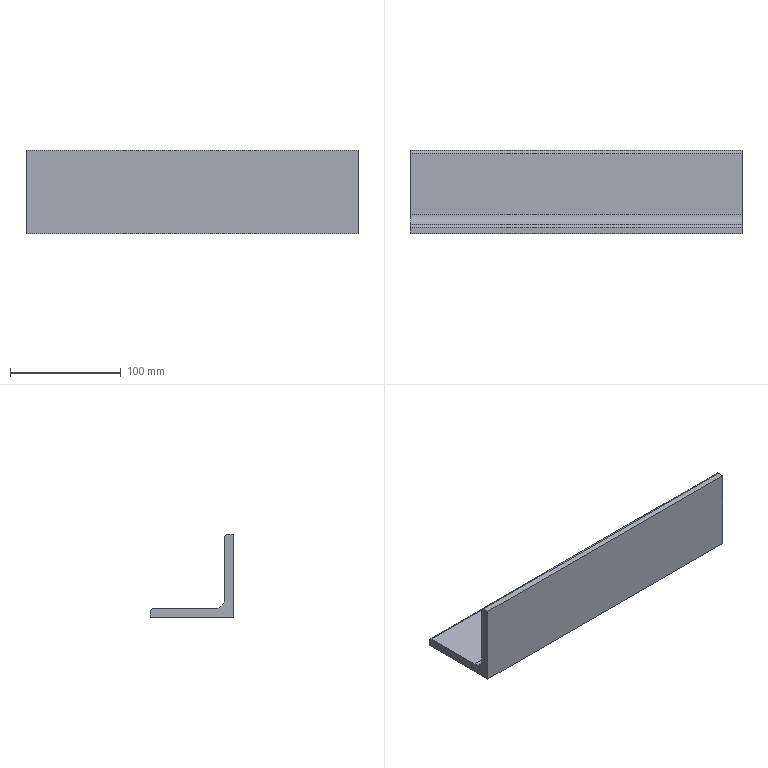Part | SolidWorks | features Extrusion 1 | 1 solid | 11 faces | box 300 x 75 x 75 mm | volume 345099 mm3 | plane 8 | cylinder 3 | commonest cylinder face diameters 5.333 x2 18 x1
STEP:
#1=CARTESIAN_POINT('',(0.,5.333,75.));
#2=VERTEX_POINT('',#1);
#3=CARTESIAN_POINT('',(0.,0.,75.));
#4=VERTEX_POINT('',#3);
#5=CARTESIAN_POINT('',(0.,0.,75.));
#6=DIRECTION('',(0.,-1.,0.));
#7=VECTOR('',#6,1000.);
#8=LINE('',#5,#7);
#9=EDGE_CURVE('',#2,#4,#8,.T.);
#10=ORIENTED_EDGE('',*,*,#9,.T.);
#11=CARTESIAN_POINT('',(300.,0.,75.));
#12=VERTEX_POINT('',#11);
#13=CARTESIAN_POINT('',(300.,0.,75.));
#14=DIRECTION('',(-1.,0.,0.));
#15=VECTOR('',#14,1000.);
#16=LINE('',#13,#15);
#17=EDGE_CURVE('',#12,#4,#16,.T.);
#18=ORIENTED_EDGE('',*,*,#17,.F.);
#19=CARTESIAN_POINT('',(300.,5.333,75.));
#20=VERTEX_POINT('',#19);
#21=CARTESIAN_POINT('',(300.,0.,75.));
#22=DIRECTION('',(0.,-1.,0.));
#23=VECTOR('',#22,1000.);
#24=LINE('',#21,#23);
#25=EDGE_CURVE('',#20,#12,#24,.T.);
#26=ORIENTED_EDGE('',*,*,#25,.F.);
#27=CARTESIAN_POINT('',(300.,5.333,75.));
#28=DIRECTION('',(-1.,0.,0.));
#29=VECTOR('',#28,1000.);
#30=LINE('',#27,#29);
#31=EDGE_CURVE('',#20,#2,#30,.T.);
#32=ORIENTED_EDGE('',*,*,#31,.T.);
#33=EDGE_LOOP('',(#10,#18,#26,#32));
#34=FACE_OUTER_BOUND('',#33,.T.);
#35=CARTESIAN_POINT('',(300.,0.,75.));
#36=DIRECTION('',(0.,0.,-1.));
#37=DIRECTION('',(-1.,0.,0.));
#38=AXIS2_PLACEMENT_3D('',#35,#36,#37);
#39=PLANE('',#38);
#40=ADVANCED_FACE('',(#34),#39,.F.);
#41=CARTESIAN_POINT('',(0.,0.,0.));
#42=VERTEX_POINT('',#41);
#43=CARTESIAN_POINT('',(0.,0.,75.));
#44=DIRECTION('',(0.,0.,-1.));
#45=VECTOR('',#44,1000.);
#46=LINE('',#43,#45);
#47=EDGE_CURVE('',#4,#42,#46,.T.);
#48=ORIENTED_EDGE('',*,*,#47,.T.);
#49=CARTESIAN_POINT('',(300.,0.,0.));
#50=VERTEX_POINT('',#49);
#51=CARTESIAN_POINT('',(300.,0.,0.));
#52=DIRECTION('',(-1.,0.,0.));
#53=VECTOR('',#52,1000.);
#54=LINE('',#51,#53);
#55=EDGE_CURVE('',#50,#42,#54,.T.);
#56=ORIENTED_EDGE('',*,*,#55,.F.);
#57=CARTESIAN_POINT('',(300.,0.,75.));
#58=DIRECTION('',(0.,0.,-1.));
#59=VECTOR('',#58,1000.);
#60=LINE('',#57,#59);
#61=EDGE_CURVE('',#12,#50,#60,.T.);
#62=ORIENTED_EDGE('',*,*,#61,.F.);
#63=ORIENTED_EDGE('',*,*,#17,.T.);
#64=EDGE_LOOP('',(#48,#56,#62,#63));
#65=FACE_OUTER_BOUND('',#64,.T.);
#66=CARTESIAN_POINT('',(300.,0.,75.));
#67=DIRECTION('',(0.,1.,0.));
#68=DIRECTION('',(0.,0.,1.));
#69=AXIS2_PLACEMENT_3D('',#66,#67,#68);
#70=PLANE('',#69);
#71=ADVANCED_FACE('',(#65),#70,.F.);
#72=CARTESIAN_POINT('',(0.,75.,0.));
#73=VERTEX_POINT('',#72);
#74=CARTESIAN_POINT('',(0.,0.,0.));
#75=DIRECTION('',(0.,1.,0.));
#76=VECTOR('',#75,1000.);
#77=LINE('',#74,#76);
#78=EDGE_CURVE('',#42,#73,#77,.T.);
#79=ORIENTED_EDGE('',*,*,#78,.T.);
#80=CARTESIAN_POINT('',(300.,75.,0.));
#81=VERTEX_POINT('',#80);
#82=CARTESIAN_POINT('',(300.,75.,0.));
#83=DIRECTION('',(-1.,0.,0.));
#84=VECTOR('',#83,1000.);
#85=LINE('',#82,#84);
#86=EDGE_CURVE('',#81,#73,#85,.T.);
#87=ORIENTED_EDGE('',*,*,#86,.F.);
#88=CARTESIAN_POINT('',(300.,0.,0.));
#89=DIRECTION('',(0.,1.,0.));
#90=VECTOR('',#89,1000.);
#91=LINE('',#88,#90);
#92=EDGE_CURVE('',#50,#81,#91,.T.);
#93=ORIENTED_EDGE('',*,*,#92,.F.);
#94=ORIENTED_EDGE('',*,*,#55,.T.);
#95=EDGE_LOOP('',(#79,#87,#93,#94));
#96=FACE_OUTER_BOUND('',#95,.T.);
#97=CARTESIAN_POINT('',(300.,0.,0.));
#98=DIRECTION('',(0.,0.,1.));
#99=DIRECTION('',(1.,0.,0.));
#100=AXIS2_PLACEMENT_3D('',#97,#98,#99);
#101=PLANE('',#100);
#102=ADVANCED_FACE('',(#96),#101,.F.);
#103=CARTESIAN_POINT('',(0.,75.,5.333));
#104=VERTEX_POINT('',#103);
#105=CARTESIAN_POINT('',(0.,75.,0.));
#106=DIRECTION('',(0.,0.,1.));
#107=VECTOR('',#106,1000.);
#108=LINE('',#105,#107);
#109=EDGE_CURVE('',#73,#104,#108,.T.);
#110=ORIENTED_EDGE('',*,*,#109,.T.);
#111=CARTESIAN_POINT('',(300.,75.,5.333));
#112=VERTEX_POINT('',#111);
#113=CARTESIAN_POINT('',(300.,75.,5.333));
#114=DIRECTION('',(-1.,0.,0.));
#115=VECTOR('',#114,1000.);
#116=LINE('',#113,#115);
#117=EDGE_CURVE('',#112,#104,#116,.T.);
#118=ORIENTED_EDGE('',*,*,#117,.F.);
#119=CARTESIAN_POINT('',(300.,75.,0.));
#120=DIRECTION('',(0.,0.,1.));
#121=VECTOR('',#120,1000.);
#122=LINE('',#119,#121);
#123=EDGE_CURVE('',#81,#112,#122,.T.);
#124=ORIENTED_EDGE('',*,*,#123,.F.);
#125=ORIENTED_EDGE('',*,*,#86,.T.);
#126=EDGE_LOOP('',(#110,#118,#124,#125));
#127=FACE_OUTER_BOUND('',#126,.T.);
#128=CARTESIAN_POINT('',(300.,75.,0.));
#129=DIRECTION('',(0.,-1.,0.));
#130=DIRECTION('',(0.,0.,-1.));
#131=AXIS2_PLACEMENT_3D('',#128,#129,#130);
#132=PLANE('',#131);
#133=ADVANCED_FACE('',(#127),#132,.F.);
#134=CARTESIAN_POINT('',(0.,72.333,8.));
#135=VERTEX_POINT('',#134);
#136=CARTESIAN_POINT('',(0.,72.333,5.333));
#137=DIRECTION('',(1.,0.,0.));
#138=DIRECTION('',(0.,0.,-1.));
#139=AXIS2_PLACEMENT_3D('',#136,#137,#138);
#140=CIRCLE('',#139,2.667);
#141=EDGE_CURVE('',#104,#135,#140,.T.);
#142=ORIENTED_EDGE('',*,*,#141,.T.);
#143=CARTESIAN_POINT('',(300.,72.333,8.));
#144=VERTEX_POINT('',#143);
#145=CARTESIAN_POINT('',(300.,72.333,8.));
#146=DIRECTION('',(-1.,0.,0.));
#147=VECTOR('',#146,1000.);
#148=LINE('',#145,#147);
#149=EDGE_CURVE('',#144,#135,#148,.T.);
#150=ORIENTED_EDGE('',*,*,#149,.F.);
#151=CARTESIAN_POINT('',(300.,72.333,5.333));
#152=DIRECTION('',(1.,0.,0.));
#153=DIRECTION('',(0.,0.,-1.));
#154=AXIS2_PLACEMENT_3D('',#151,#152,#153);
#155=CIRCLE('',#154,2.667);
#156=EDGE_CURVE('',#112,#144,#155,.T.);
#157=ORIENTED_EDGE('',*,*,#156,.F.);
#158=ORIENTED_EDGE('',*,*,#117,.T.);
#159=EDGE_LOOP('',(#142,#150,#157,#158));
#160=FACE_OUTER_BOUND('',#159,.T.);
#161=CARTESIAN_POINT('',(300.,72.333,5.333));
#162=DIRECTION('',(-1.,0.,0.));
#163=DIRECTION('',(0.,0.,1.));
#164=AXIS2_PLACEMENT_3D('',#161,#162,#163);
#165=CYLINDRICAL_SURFACE('',#164,2.667);
#166=ADVANCED_FACE('',(#160),#165,.T.);
#167=CARTESIAN_POINT('',(0.,17.,8.));
#168=VERTEX_POINT('',#167);
#169=CARTESIAN_POINT('',(0.,17.,8.));
#170=DIRECTION('',(0.,-1.,0.));
#171=VECTOR('',#170,1000.);
#172=LINE('',#169,#171);
#173=EDGE_CURVE('',#135,#168,#172,.T.);
#174=ORIENTED_EDGE('',*,*,#173,.T.);
#175=CARTESIAN_POINT('',(300.,17.,8.));
#176=VERTEX_POINT('',#175);
#177=CARTESIAN_POINT('',(300.,17.,8.));
#178=DIRECTION('',(-1.,0.,0.));
#179=VECTOR('',#178,1000.);
#180=LINE('',#177,#179);
#181=EDGE_CURVE('',#176,#168,#180,.T.);
#182=ORIENTED_EDGE('',*,*,#181,.F.);
#183=CARTESIAN_POINT('',(300.,17.,8.));
#184=DIRECTION('',(0.,-1.,0.));
#185=VECTOR('',#184,1000.);
#186=LINE('',#183,#185);
#187=EDGE_CURVE('',#144,#176,#186,.T.);
#188=ORIENTED_EDGE('',*,*,#187,.F.);
#189=ORIENTED_EDGE('',*,*,#149,.T.);
#190=EDGE_LOOP('',(#174,#182,#188,#189));
#191=FACE_OUTER_BOUND('',#190,.T.);
#192=CARTESIAN_POINT('',(300.,17.,8.));
#193=DIRECTION('',(0.,0.,-1.));
#194=DIRECTION('',(-1.,0.,0.));
#195=AXIS2_PLACEMENT_3D('',#192,#193,#194);
#196=PLANE('',#195);
#197=ADVANCED_FACE('',(#191),#196,.F.);
#198=CARTESIAN_POINT('',(0.,8.,17.));
#199=VERTEX_POINT('',#198);
#200=CARTESIAN_POINT('',(0.,17.,17.));
#201=DIRECTION('',(-1.,0.,0.));
#202=DIRECTION('',(0.,0.,-1.));
#203=AXIS2_PLACEMENT_3D('',#200,#201,#202);
#204=CIRCLE('',#203,9.);
#205=EDGE_CURVE('',#168,#199,#204,.T.);
#206=ORIENTED_EDGE('',*,*,#205,.T.);
#207=CARTESIAN_POINT('',(300.,8.,17.));
#208=VERTEX_POINT('',#207);
#209=CARTESIAN_POINT('',(300.,8.,17.));
#210=DIRECTION('',(-1.,0.,0.));
#211=VECTOR('',#210,1000.);
#212=LINE('',#209,#211);
#213=EDGE_CURVE('',#208,#199,#212,.T.);
#214=ORIENTED_EDGE('',*,*,#213,.F.);
#215=CARTESIAN_POINT('',(300.,17.,17.));
#216=DIRECTION('',(-1.,0.,0.));
#217=DIRECTION('',(0.,0.,-1.));
#218=AXIS2_PLACEMENT_3D('',#215,#216,#217);
#219=CIRCLE('',#218,9.);
#220=EDGE_CURVE('',#176,#208,#219,.T.);
#221=ORIENTED_EDGE('',*,*,#220,.F.);
#222=ORIENTED_EDGE('',*,*,#181,.T.);
#223=EDGE_LOOP('',(#206,#214,#221,#222));
#224=FACE_OUTER_BOUND('',#223,.T.);
#225=CARTESIAN_POINT('',(300.,17.,17.));
#226=DIRECTION('',(-1.,0.,0.));
#227=DIRECTION('',(0.,0.,1.));
#228=AXIS2_PLACEMENT_3D('',#225,#226,#227);
#229=CYLINDRICAL_SURFACE('',#228,9.);
#230=ADVANCED_FACE('',(#224),#229,.F.);
#231=CARTESIAN_POINT('',(0.,8.,72.333));
#232=VERTEX_POINT('',#231);
#233=CARTESIAN_POINT('',(0.,8.,72.333));
#234=DIRECTION('',(0.,0.,1.));
#235=VECTOR('',#234,1000.);
#236=LINE('',#233,#235);
#237=EDGE_CURVE('',#199,#232,#236,.T.);
#238=ORIENTED_EDGE('',*,*,#237,.T.);
#239=CARTESIAN_POINT('',(300.,8.,72.333));
#240=VERTEX_POINT('',#239);
#241=CARTESIAN_POINT('',(300.,8.,72.333));
#242=DIRECTION('',(-1.,0.,0.));
#243=VECTOR('',#242,1000.);
#244=LINE('',#241,#243);
#245=EDGE_CURVE('',#240,#232,#244,.T.);
#246=ORIENTED_EDGE('',*,*,#245,.F.);
#247=CARTESIAN_POINT('',(300.,8.,72.333));
#248=DIRECTION('',(0.,0.,1.));
#249=VECTOR('',#248,1000.);
#250=LINE('',#247,#249);
#251=EDGE_CURVE('',#208,#240,#250,.T.);
#252=ORIENTED_EDGE('',*,*,#251,.F.);
#253=ORIENTED_EDGE('',*,*,#213,.T.);
#254=EDGE_LOOP('',(#238,#246,#252,#253));
#255=FACE_OUTER_BOUND('',#254,.T.);
#256=CARTESIAN_POINT('',(300.,8.,72.333));
#257=DIRECTION('',(0.,-1.,0.));
#258=DIRECTION('',(0.,0.,-1.));
#259=AXIS2_PLACEMENT_3D('',#256,#257,#258);
#260=PLANE('',#259);
#261=ADVANCED_FACE('',(#255),#260,.F.);
#262=CARTESIAN_POINT('',(0.,5.333,72.333));
#263=DIRECTION('',(1.,0.,0.));
#264=DIRECTION('',(0.,0.,1.));
#265=AXIS2_PLACEMENT_3D('',#262,#263,#264);
#266=CIRCLE('',#265,2.667);
#267=EDGE_CURVE('',#232,#2,#266,.T.);
#268=ORIENTED_EDGE('',*,*,#267,.T.);
#269=ORIENTED_EDGE('',*,*,#31,.F.);
#270=CARTESIAN_POINT('',(300.,5.333,72.333));
#271=DIRECTION('',(1.,0.,0.));
#272=DIRECTION('',(0.,0.,1.));
#273=AXIS2_PLACEMENT_3D('',#270,#271,#272);
#274=CIRCLE('',#273,2.667);
#275=EDGE_CURVE('',#240,#20,#274,.T.);
#276=ORIENTED_EDGE('',*,*,#275,.F.);
#277=ORIENTED_EDGE('',*,*,#245,.T.);
#278=EDGE_LOOP('',(#268,#269,#276,#277));
#279=FACE_OUTER_BOUND('',#278,.T.);
#280=CARTESIAN_POINT('',(300.,5.333,72.333));
#281=DIRECTION('',(-1.,0.,0.));
#282=DIRECTION('',(0.,0.,1.));
#283=AXIS2_PLACEMENT_3D('',#280,#281,#282);
#284=CYLINDRICAL_SURFACE('',#283,2.667);
#285=ADVANCED_FACE('',(#279),#284,.T.);
#286=ORIENTED_EDGE('',*,*,#25,.T.);
#287=ORIENTED_EDGE('',*,*,#61,.T.);
#288=ORIENTED_EDGE('',*,*,#92,.T.);
#289=ORIENTED_EDGE('',*,*,#123,.T.);
#290=ORIENTED_EDGE('',*,*,#156,.T.);
#291=ORIENTED_EDGE('',*,*,#187,.T.);
#292=ORIENTED_EDGE('',*,*,#220,.T.);
#293=ORIENTED_EDGE('',*,*,#251,.T.);
#294=ORIENTED_EDGE('',*,*,#275,.T.);
#295=EDGE_LOOP('',(#286,#287,#288,#289,#290,#291,#292,#293,#294));
#296=FACE_OUTER_BOUND('',#295,.T.);
#297=CARTESIAN_POINT('',(300.,5.333,72.333));
#298=DIRECTION('',(-1.,0.,0.));
#299=DIRECTION('',(0.,0.,1.));
#300=AXIS2_PLACEMENT_3D('',#297,#298,#299);
#301=PLANE('',#300);
#302=ADVANCED_FACE('',(#296),#301,.F.);
#303=ORIENTED_EDGE('',*,*,#9,.F.);
#304=ORIENTED_EDGE('',*,*,#267,.F.);
#305=ORIENTED_EDGE('',*,*,#237,.F.);
#306=ORIENTED_EDGE('',*,*,#205,.F.);
#307=ORIENTED_EDGE('',*,*,#173,.F.);
#308=ORIENTED_EDGE('',*,*,#141,.F.);
#309=ORIENTED_EDGE('',*,*,#109,.F.);
#310=ORIENTED_EDGE('',*,*,#78,.F.);
#311=ORIENTED_EDGE('',*,*,#47,.F.);
#312=EDGE_LOOP('',(#303,#304,#305,#306,#307,#308,#309,#310,#311));
#313=FACE_OUTER_BOUND('',#312,.T.);
#314=CARTESIAN_POINT('',(0.,5.333,72.333));
#315=DIRECTION('',(-1.,0.,0.));
#316=DIRECTION('',(0.,0.,1.));
#317=AXIS2_PLACEMENT_3D('',#314,#315,#316);
#318=PLANE('',#317);
#319=ADVANCED_FACE('',(#313),#318,.T.);
#320=CLOSED_SHELL('',(#40,#71,#102,#133,#166,#197,#230,#261,#285,#302,#319));
#321=MANIFOLD_SOLID_BREP('',#320);
#322=CARTESIAN_POINT('',(0.,0.,0.));
#323=DIRECTION('',(0.,0.,1.));
#324=DIRECTION('',(1.,0.,0.));
#325=AXIS2_PLACEMENT_3D('',#322,#323,#324);
#326=(LENGTH_UNIT()NAMED_UNIT(*)SI_UNIT(.MILLI.,.METRE.));
#327=UNCERTAINTY_MEASURE_WITH_UNIT(LENGTH_MEASURE(0.00001),#326,'','');
#328=(NAMED_UNIT(*)PLANE_ANGLE_UNIT()SI_UNIT($,.RADIAN.));
#329=(NAMED_UNIT(*)SI_UNIT($,.STERADIAN.)SOLID_ANGLE_UNIT());
#330=(GEOMETRIC_REPRESENTATION_CONTEXT(3)GLOBAL_UNCERTAINTY_ASSIGNED_CONTEXT((#327))GLOBAL_UNIT_ASSIGNED_CONTEXT((#326,#328,#329))REPRESENTATION_CONTEXT('',''));
#331=ADVANCED_BREP_SHAPE_REPRESENTATION('',(#321,#325),#330);